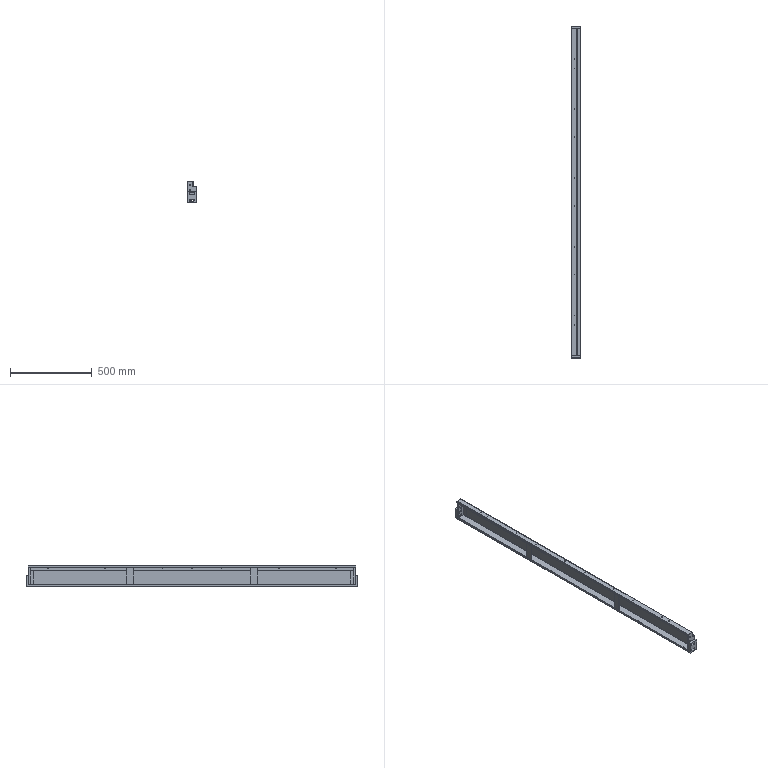Part | 7 solids | 254 faces | box 58 x 2030 x 130 mm | volume 770798 mm3 | plane 142 | cylinder 112 | commonest cylinder face diameters 5 x32 11 x32 9 x18 4.6 x14 2 x10 4.4 x6